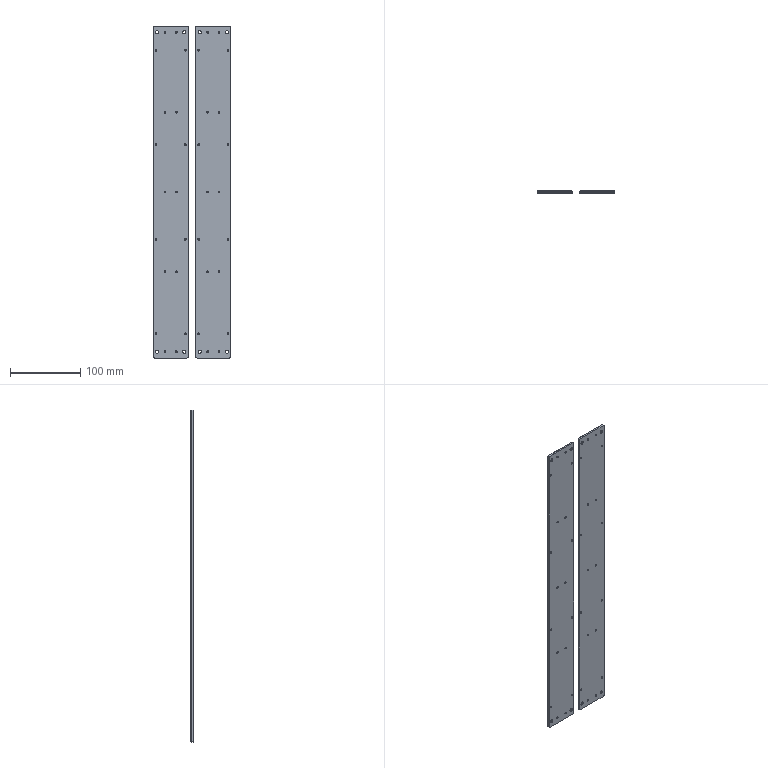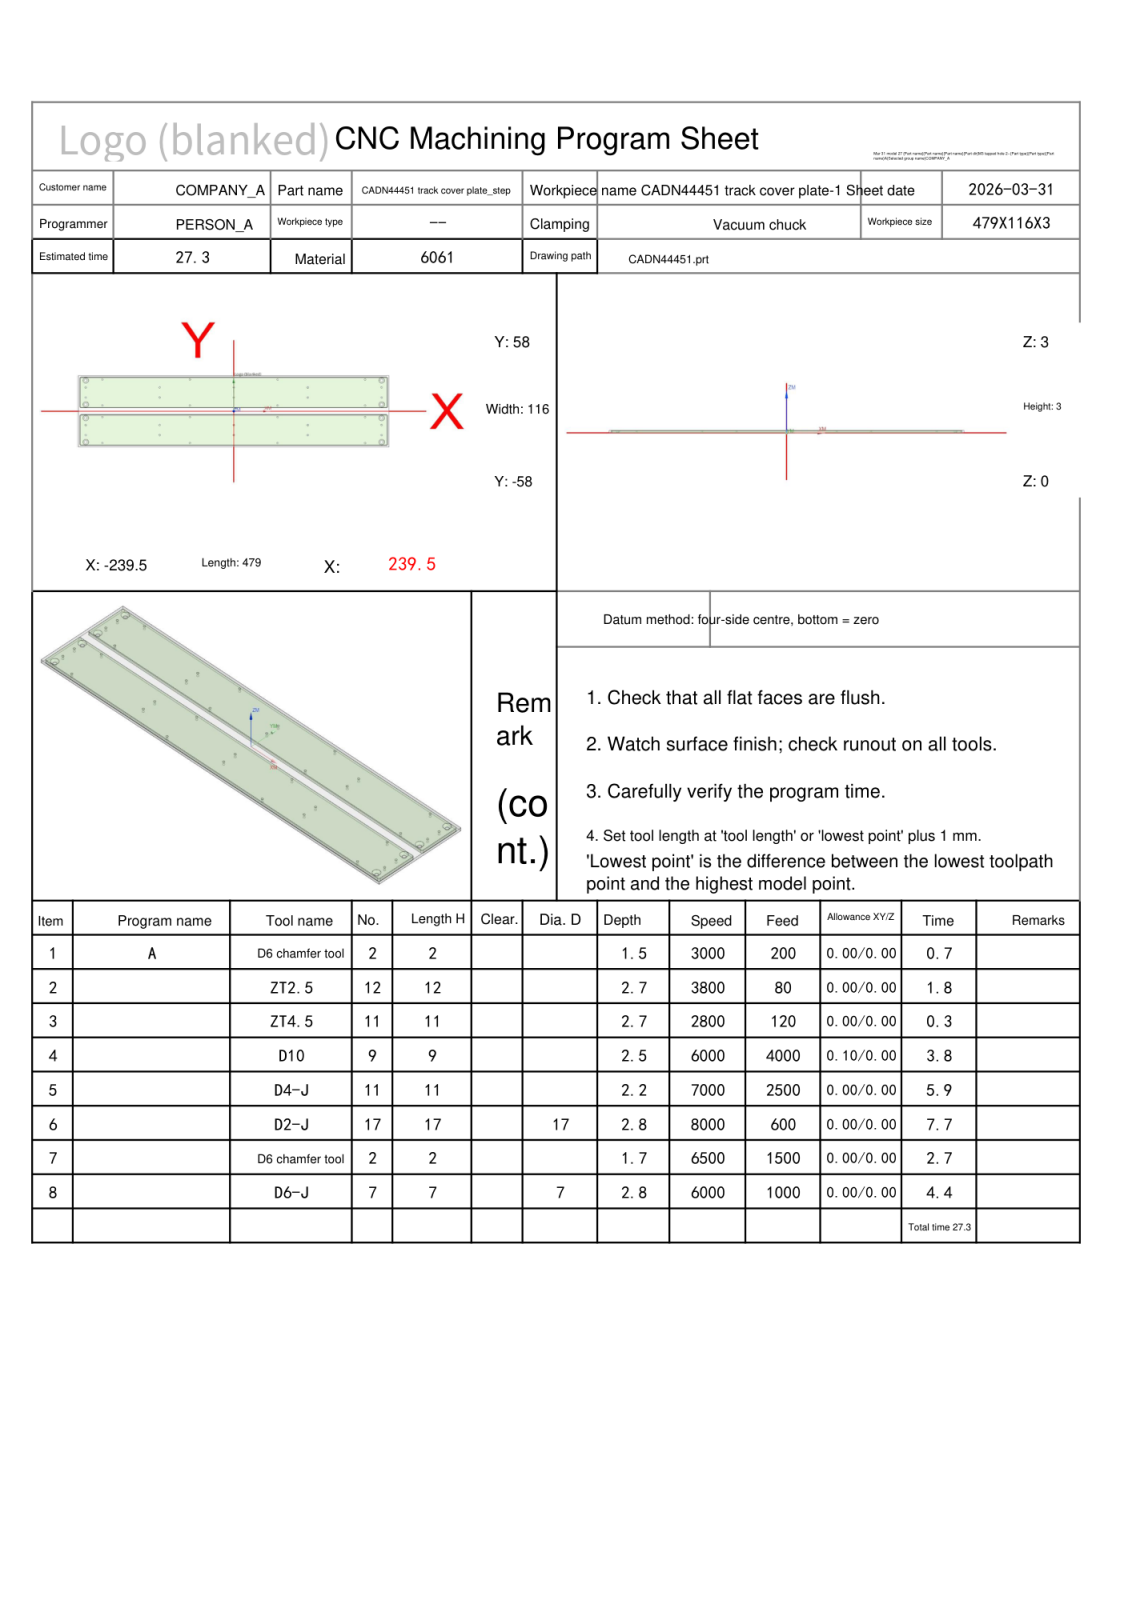NC program | NX | posted by the shop | part box 111 x 3 x 474 mm
Lines 17823 to 17996 of 17996:
N7 T02 M06
(D6 chamfer tool  D=6. R=0. H=02 ce=0.00 di=0.00)
G00 G90 G54 X202.5 Y51.5 M03 S5000
G43 H02 Z23.
M08
G98 G81 X202.5 Y51.5 Z1.25 R6. F150.
X228. Y38.6
Y22.4
X202.5 Y9.5
Y-9.5
X228. Y-22.4
Y-38.6
X202.5 Y-51.5
X114. Y-38.6
Y-22.4
Y22.4
Y38.6
X67.5 Y51.5
Y9.5
Y-9.5
Y-51.5
X0.0 Y-38.6
Y-22.4
Y22.4
Y38.6
X-67.5 Y51.5
Y9.5
Y-9.5
Y-51.5
X-114. Y-38.6
Y-22.4
Y22.4
Y38.6
X-202.5 Y51.5
X-228. Y38.6
Y22.4
X-202.5 Y9.5
Y-9.5
X-228. Y-22.4
Y-38.6
X-202.5 Y-51.5
G80
G00 Z23.
G00 G90 X-236.186 Y57.215 M03 S6500
Z23.
Z3.3
G01 Z1.8 F1500.
G03 X-235. Y56.2 I1.186 J.185
G01 X235.
G02 X237.438 Y54.66 I0.0 J-2.7
X237.538 Y54.421 I-2.438 J-1.16
X237.681 Y53.824 I-2.538 J-.921
X237.7 Y53.5 I-2.681 J-.324
G01 Y7.5
G02 X235. Y4.8 I-2.7 J0.0
G01 X-235.
G02 X-237.7 Y7.5 I0.0 J2.7
G01 Y53.5
G02 X-235. Y56.2 I2.7 J0.0
G01 X-234.6
G03 X-233.4 Y57.4 I0.0 J1.2
G01 Z3.3
G00 Z23.
X1.2 Y-57.4
Z3.3
G01 Z1.8
G03 X0.0 Y-56.2 I-1.2 J0.0
G01 X-235.
G02 X-237.7 Y-53.5 I0.0 J2.7
G01 Y-7.5
G02 X-235. Y-4.8 I2.7 J0.0
G01 X235.
G02 X237.696 Y-7.355 I0.0 J-2.7
G01 X237.702 Y-7.427
X237.7 Y-7.5
Y-53.5
G02 X235. Y-56.2 I-2.7 J0.0
G01 X0.0
X-.4
G03 X-1.6 Y-57.4 I0.0 J-1.2
G01 Z3.3
G00 Z23.
G91 G28 Z0.0
M05
M09
G91 G28 Z0.0
M01
N8 T07 M06
(D6-J  D=6. R=0. H=07 ce=0.00 di=0.00)
G00 G90 G54 X236.013 Y-59.616 M03 S6000
G43 H07 Z23.
M08
Z1.
G01 Z.5 F1000.
G41 D07
X235.997 Y-59.417
G03 X235. Y-58.5 I-.997 J-.083
G01 X-235.
G02 X-240. Y-53.5 I0.0 J5.
G01 Y-7.5
G02 X-235. Y-2.5 I5. J0.0
G01 X235.
G02 X240. Y-7.5 I0.0 J-5.
G01 Y-53.5
G02 X235. Y-58.5 I-5. J0.0
G01 X234.5
G03 X233.5 Y-59.5 I0.0 J-1.
G01 G40 Y-59.7
Z1.
G00 Z23.
X-236.013 Y59.616
Z1.
G01 Z.5
G41 D07
X-235.997 Y59.417
G03 X-235. Y58.5 I.997 J.083
G01 X235.
G02 X240. Y53.5 I0.0 J-5.
G01 Y7.5
G02 X235. Y2.5 I-5. J0.0
G01 X-235.
G02 X-240. Y7.5 I0.0 J5.
G01 Y53.5
G02 X-235. Y58.5 I5. J0.0
G01 X-234.5
G03 X-233.5 Y59.5 I0.0 J1.
G01 G40 Y59.7
Z1.
G00 Z23.
G00 G90 X236.005 Y-59.516 M03 S6000
Z23.
Z.7
G01 Z.2 F1000.
G41 D07
X235.997 Y-59.417
G03 X235. Y-58.5 I-.997 J-.083
G01 X-235.
G02 X-240. Y-53.5 I0.0 J5.
G01 Y-7.5
G02 X-235. Y-2.5 I5. J0.0
G01 X235.
G02 X240. Y-7.5 I0.0 J-5.
G01 Y-53.5
G02 X235. Y-58.5 I-5. J0.0
G01 X234.5
G03 X233.5 Y-59.5 I0.0 J-1.
G01 G40 Y-59.6
Z.7
G00 Z23.
X-236.005 Y59.516
Z.7
G01 Z.2
G41 D07
X-235.997 Y59.417
G03 X-235. Y58.5 I.997 J.083
G01 X235.
G02 X240. Y53.5 I0.0 J-5.
G01 Y7.5
G02 X235. Y2.5 I-5. J0.0
G01 X-235.
G02 X-240. Y7.5 I0.0 J5.
G01 Y53.5
G02 X-235. Y58.5 I5. J0.0
G01 X-234.5
G03 X-233.5 Y59.5 I0.0 J1.
G01 G40 Y59.6
Z.7
G00 Z23.
M05
M09
G91 G28 Z0.0
G91 G28 Y0.0
M30
%